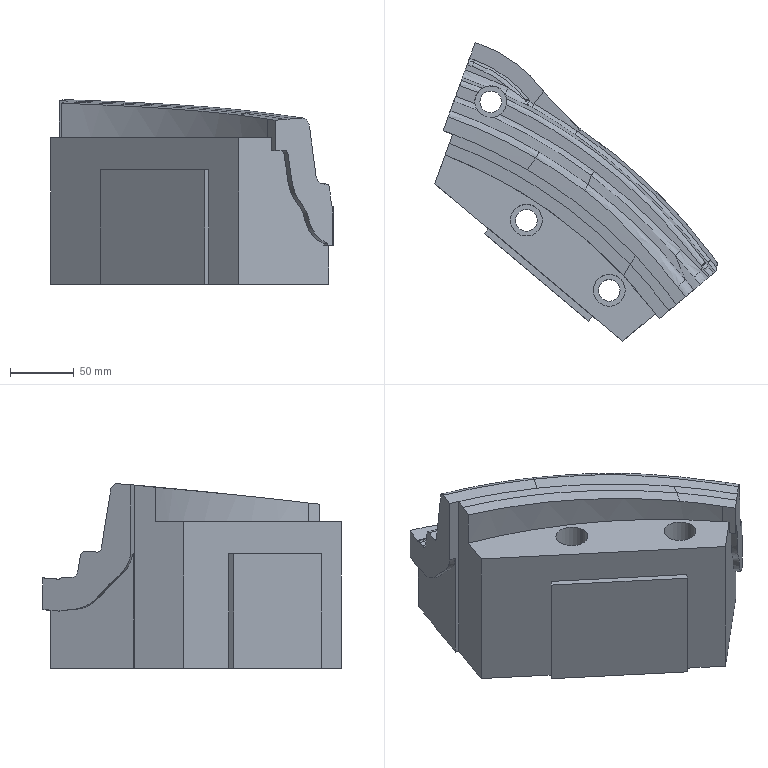Part | NX | features solid 2 | 1 solid | 90 faces | box 221.692 x 234.359 x 144.94 mm | volume 2557729 mm3 | spline 59 | plane 20 | cylinder 11 | commonest cylinder face diameters 17 x3 25 x3 6 x2 10 x1 11.917 x1 183.4 x1